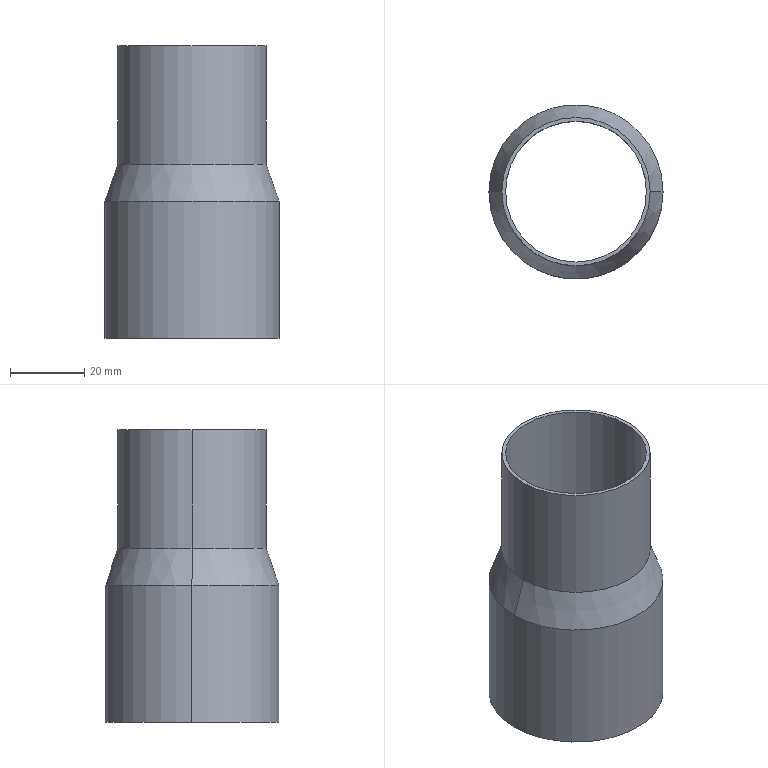Part | SolidWorks | features 3DProfileFeature 2, ICE 2, NetBlend 1, NetBlendCut 1 | 1 solid | 14 faces | box 47 x 47 x 79 mm | volume 10603 mm3 | cylinder 8 | cone 4 | plane 2 | commonest cylinder face diameters 38 x2 40 x2 45 x2 47 x2
STEP:
#1=CARTESIAN_POINT('',(-19.,0.,42.));
#2=VERTEX_POINT('',#1);
#3=CARTESIAN_POINT('',(19.,0.,42.));
#4=VERTEX_POINT('',#3);
#5=CARTESIAN_POINT('',(0.,0.,42.));
#6=DIRECTION('',(0.,0.,1.));
#7=DIRECTION('',(1.,0.,0.));
#8=AXIS2_PLACEMENT_3D('',#5,#6,#7);
#9=CIRCLE('',#8,19.);
#10=EDGE_CURVE('',#2,#4,#9,.T.);
#11=ORIENTED_EDGE('',*,*,#10,.T.);
#12=CARTESIAN_POINT('',(19.,0.,10.));
#13=VERTEX_POINT('',#12);
#14=CARTESIAN_POINT('',(19.,0.,42.));
#15=DIRECTION('',(0.,0.,-1.));
#16=VECTOR('',#15,1000.);
#17=LINE('',#14,#16);
#18=EDGE_CURVE('',#4,#13,#17,.T.);
#19=ORIENTED_EDGE('',*,*,#18,.T.);
#20=CARTESIAN_POINT('',(-19.,0.,10.));
#21=VERTEX_POINT('',#20);
#22=CARTESIAN_POINT('',(0.,0.,10.));
#23=DIRECTION('',(0.,0.,-1.));
#24=DIRECTION('',(1.,0.,0.));
#25=AXIS2_PLACEMENT_3D('',#22,#23,#24);
#26=CIRCLE('',#25,19.);
#27=EDGE_CURVE('',#13,#21,#26,.T.);
#28=ORIENTED_EDGE('',*,*,#27,.T.);
#29=CARTESIAN_POINT('',(-19.,0.,42.));
#30=DIRECTION('',(0.,0.,-1.));
#31=VECTOR('',#30,1000.);
#32=LINE('',#29,#31);
#33=EDGE_CURVE('',#2,#21,#32,.T.);
#34=ORIENTED_EDGE('',*,*,#33,.F.);
#35=EDGE_LOOP('',(#11,#19,#28,#34));
#36=FACE_OUTER_BOUND('',#35,.T.);
#37=CARTESIAN_POINT('',(0.,0.,42.));
#38=DIRECTION('',(0.,0.,-1.));
#39=DIRECTION('',(-1.,0.,0.));
#40=AXIS2_PLACEMENT_3D('',#37,#38,#39);
#41=CYLINDRICAL_SURFACE('',#40,19.);
#42=ADVANCED_FACE('',(#36),#41,.F.);
#43=CARTESIAN_POINT('',(20.,0.,42.));
#44=VERTEX_POINT('',#43);
#45=CARTESIAN_POINT('',(-20.,0.,42.));
#46=VERTEX_POINT('',#45);
#47=CARTESIAN_POINT('',(0.,0.,42.));
#48=DIRECTION('',(0.,0.,1.));
#49=DIRECTION('',(1.,0.,0.));
#50=AXIS2_PLACEMENT_3D('',#47,#48,#49);
#51=CIRCLE('',#50,20.);
#52=EDGE_CURVE('',#44,#46,#51,.T.);
#53=ORIENTED_EDGE('',*,*,#52,.F.);
#54=CARTESIAN_POINT('',(20.,0.,10.));
#55=VERTEX_POINT('',#54);
#56=CARTESIAN_POINT('',(20.,0.,42.));
#57=DIRECTION('',(0.,0.,-1.));
#58=VECTOR('',#57,1000.);
#59=LINE('',#56,#58);
#60=EDGE_CURVE('',#44,#55,#59,.T.);
#61=ORIENTED_EDGE('',*,*,#60,.T.);
#62=CARTESIAN_POINT('',(-20.,0.,10.));
#63=VERTEX_POINT('',#62);
#64=CARTESIAN_POINT('',(0.,0.,10.));
#65=DIRECTION('',(0.,0.,1.));
#66=DIRECTION('',(1.,0.,0.));
#67=AXIS2_PLACEMENT_3D('',#64,#65,#66);
#68=CIRCLE('',#67,20.);
#69=EDGE_CURVE('',#55,#63,#68,.T.);
#70=ORIENTED_EDGE('',*,*,#69,.T.);
#71=CARTESIAN_POINT('',(-20.,0.,42.));
#72=DIRECTION('',(0.,0.,-1.));
#73=VECTOR('',#72,1000.);
#74=LINE('',#71,#73);
#75=EDGE_CURVE('',#46,#63,#74,.T.);
#76=ORIENTED_EDGE('',*,*,#75,.F.);
#77=EDGE_LOOP('',(#53,#61,#70,#76));
#78=FACE_OUTER_BOUND('',#77,.T.);
#79=CARTESIAN_POINT('',(0.,0.,42.));
#80=DIRECTION('',(0.,0.,-1.));
#81=DIRECTION('',(-1.,0.,0.));
#82=AXIS2_PLACEMENT_3D('',#79,#80,#81);
#83=CYLINDRICAL_SURFACE('',#82,20.);
#84=ADVANCED_FACE('',(#78),#83,.T.);
#85=CARTESIAN_POINT('',(22.5,0.,-37.));
#86=VERTEX_POINT('',#85);
#87=CARTESIAN_POINT('',(-22.5,0.,-37.));
#88=VERTEX_POINT('',#87);
#89=CARTESIAN_POINT('',(0.,0.,-37.));
#90=DIRECTION('',(0.,0.,-1.));
#91=DIRECTION('',(-1.,0.,0.));
#92=AXIS2_PLACEMENT_3D('',#89,#90,#91);
#93=CIRCLE('',#92,22.5);
#94=EDGE_CURVE('',#86,#88,#93,.T.);
#95=ORIENTED_EDGE('',*,*,#94,.T.);
#96=CARTESIAN_POINT('',(-22.5,0.,0.));
#97=VERTEX_POINT('',#96);
#98=CARTESIAN_POINT('',(-22.5,0.,-37.));
#99=DIRECTION('',(0.,0.,1.));
#100=VECTOR('',#99,1000.);
#101=LINE('',#98,#100);
#102=EDGE_CURVE('',#88,#97,#101,.T.);
#103=ORIENTED_EDGE('',*,*,#102,.T.);
#104=CARTESIAN_POINT('',(22.5,0.,0.));
#105=VERTEX_POINT('',#104);
#106=CARTESIAN_POINT('',(0.,0.,0.));
#107=DIRECTION('',(0.,0.,-1.));
#108=DIRECTION('',(-1.,0.,0.));
#109=AXIS2_PLACEMENT_3D('',#106,#107,#108);
#110=CIRCLE('',#109,22.5);
#111=EDGE_CURVE('',#105,#97,#110,.T.);
#112=ORIENTED_EDGE('',*,*,#111,.F.);
#113=CARTESIAN_POINT('',(22.5,0.,-37.));
#114=DIRECTION('',(0.,0.,1.));
#115=VECTOR('',#114,1000.);
#116=LINE('',#113,#115);
#117=EDGE_CURVE('',#86,#105,#116,.T.);
#118=ORIENTED_EDGE('',*,*,#117,.F.);
#119=EDGE_LOOP('',(#95,#103,#112,#118));
#120=FACE_OUTER_BOUND('',#119,.T.);
#121=CARTESIAN_POINT('',(0.,0.,-37.));
#122=DIRECTION('',(0.,0.,1.));
#123=DIRECTION('',(1.,0.,0.));
#124=AXIS2_PLACEMENT_3D('',#121,#122,#123);
#125=CYLINDRICAL_SURFACE('',#124,22.5);
#126=ADVANCED_FACE('',(#120),#125,.F.);
#127=CARTESIAN_POINT('',(-23.5,0.,-37.));
#128=VERTEX_POINT('',#127);
#129=CARTESIAN_POINT('',(23.5,0.,-37.));
#130=VERTEX_POINT('',#129);
#131=CARTESIAN_POINT('',(0.,0.,-37.));
#132=DIRECTION('',(0.,0.,-1.));
#133=DIRECTION('',(-1.,0.,0.));
#134=AXIS2_PLACEMENT_3D('',#131,#132,#133);
#135=CIRCLE('',#134,23.5);
#136=EDGE_CURVE('',#128,#130,#135,.T.);
#137=ORIENTED_EDGE('',*,*,#136,.F.);
#138=CARTESIAN_POINT('',(-23.5,0.,0.));
#139=VERTEX_POINT('',#138);
#140=CARTESIAN_POINT('',(-23.5,0.,-37.));
#141=DIRECTION('',(0.,0.,1.));
#142=VECTOR('',#141,1000.);
#143=LINE('',#140,#142);
#144=EDGE_CURVE('',#128,#139,#143,.T.);
#145=ORIENTED_EDGE('',*,*,#144,.T.);
#146=CARTESIAN_POINT('',(23.5,0.,0.));
#147=VERTEX_POINT('',#146);
#148=CARTESIAN_POINT('',(0.,0.,0.));
#149=DIRECTION('',(0.,0.,-1.));
#150=DIRECTION('',(-1.,0.,0.));
#151=AXIS2_PLACEMENT_3D('',#148,#149,#150);
#152=CIRCLE('',#151,23.5);
#153=EDGE_CURVE('',#139,#147,#152,.T.);
#154=ORIENTED_EDGE('',*,*,#153,.T.);
#155=CARTESIAN_POINT('',(23.5,0.,-37.));
#156=DIRECTION('',(0.,0.,1.));
#157=VECTOR('',#156,1000.);
#158=LINE('',#155,#157);
#159=EDGE_CURVE('',#130,#147,#158,.T.);
#160=ORIENTED_EDGE('',*,*,#159,.F.);
#161=EDGE_LOOP('',(#137,#145,#154,#160));
#162=FACE_OUTER_BOUND('',#161,.T.);
#163=CARTESIAN_POINT('',(0.,0.,-37.));
#164=DIRECTION('',(0.,0.,1.));
#165=DIRECTION('',(1.,0.,0.));
#166=AXIS2_PLACEMENT_3D('',#163,#164,#165);
#167=CYLINDRICAL_SURFACE('',#166,23.5);
#168=ADVANCED_FACE('',(#162),#167,.T.);
#169=ORIENTED_EDGE('',*,*,#27,.F.);
#170=CARTESIAN_POINT('',(19.,0.,10.));
#171=DIRECTION('',(0.3304,0.,-0.9439));
#172=VECTOR('',#171,1000.);
#173=LINE('',#170,#172);
#174=EDGE_CURVE('',#13,#105,#173,.T.);
#175=ORIENTED_EDGE('',*,*,#174,.T.);
#176=ORIENTED_EDGE('',*,*,#111,.T.);
#177=CARTESIAN_POINT('',(-19.,0.,10.));
#178=DIRECTION('',(-0.3304,0.,-0.9439));
#179=VECTOR('',#178,1000.);
#180=LINE('',#177,#179);
#181=EDGE_CURVE('',#21,#97,#180,.T.);
#182=ORIENTED_EDGE('',*,*,#181,.F.);
#183=EDGE_LOOP('',(#169,#175,#176,#182));
#184=FACE_OUTER_BOUND('',#183,.T.);
#185=CARTESIAN_POINT('',(0.,0.,10.));
#186=DIRECTION('',(0.,0.,-1.));
#187=DIRECTION('',(-1.,0.,0.));
#188=AXIS2_PLACEMENT_3D('',#185,#186,#187);
#189=CONICAL_SURFACE('',#188,19.,0.3367);
#190=ADVANCED_FACE('',(#184),#189,.F.);
#191=ORIENTED_EDGE('',*,*,#69,.F.);
#192=CARTESIAN_POINT('',(20.,0.,10.));
#193=DIRECTION('',(0.3304,0.,-0.9439));
#194=VECTOR('',#193,1000.);
#195=LINE('',#192,#194);
#196=EDGE_CURVE('',#55,#147,#195,.T.);
#197=ORIENTED_EDGE('',*,*,#196,.T.);
#198=ORIENTED_EDGE('',*,*,#153,.F.);
#199=CARTESIAN_POINT('',(-20.,0.,10.));
#200=DIRECTION('',(-0.3304,0.,-0.9439));
#201=VECTOR('',#200,1000.);
#202=LINE('',#199,#201);
#203=EDGE_CURVE('',#63,#139,#202,.T.);
#204=ORIENTED_EDGE('',*,*,#203,.F.);
#205=EDGE_LOOP('',(#191,#197,#198,#204));
#206=FACE_OUTER_BOUND('',#205,.T.);
#207=CARTESIAN_POINT('',(0.,0.,10.));
#208=DIRECTION('',(0.,0.,-1.));
#209=DIRECTION('',(-1.,0.,0.));
#210=AXIS2_PLACEMENT_3D('',#207,#208,#209);
#211=CONICAL_SURFACE('',#210,20.,0.3367);
#212=ADVANCED_FACE('',(#206),#211,.T.);
#213=ORIENTED_EDGE('',*,*,#196,.F.);
#214=CARTESIAN_POINT('',(0.,0.,10.));
#215=DIRECTION('',(0.,0.,1.));
#216=DIRECTION('',(1.,0.,0.));
#217=AXIS2_PLACEMENT_3D('',#214,#215,#216);
#218=CIRCLE('',#217,20.);
#219=EDGE_CURVE('',#63,#55,#218,.T.);
#220=ORIENTED_EDGE('',*,*,#219,.F.);
#221=ORIENTED_EDGE('',*,*,#203,.T.);
#222=CARTESIAN_POINT('',(0.,0.,0.));
#223=DIRECTION('',(0.,0.,-1.));
#224=DIRECTION('',(-1.,0.,0.));
#225=AXIS2_PLACEMENT_3D('',#222,#223,#224);
#226=CIRCLE('',#225,23.5);
#227=EDGE_CURVE('',#147,#139,#226,.T.);
#228=ORIENTED_EDGE('',*,*,#227,.F.);
#229=EDGE_LOOP('',(#213,#220,#221,#228));
#230=FACE_OUTER_BOUND('',#229,.T.);
#231=CARTESIAN_POINT('',(0.,0.,10.));
#232=DIRECTION('',(0.,0.,-1.));
#233=DIRECTION('',(-1.,0.,0.));
#234=AXIS2_PLACEMENT_3D('',#231,#232,#233);
#235=CONICAL_SURFACE('',#234,20.,0.3367);
#236=ADVANCED_FACE('',(#230),#235,.T.);
#237=ORIENTED_EDGE('',*,*,#174,.F.);
#238=CARTESIAN_POINT('',(0.,0.,10.));
#239=DIRECTION('',(0.,0.,-1.));
#240=DIRECTION('',(1.,0.,0.));
#241=AXIS2_PLACEMENT_3D('',#238,#239,#240);
#242=CIRCLE('',#241,19.);
#243=EDGE_CURVE('',#21,#13,#242,.T.);
#244=ORIENTED_EDGE('',*,*,#243,.F.);
#245=ORIENTED_EDGE('',*,*,#181,.T.);
#246=CARTESIAN_POINT('',(0.,0.,0.));
#247=DIRECTION('',(0.,0.,-1.));
#248=DIRECTION('',(-1.,0.,0.));
#249=AXIS2_PLACEMENT_3D('',#246,#247,#248);
#250=CIRCLE('',#249,22.5);
#251=EDGE_CURVE('',#97,#105,#250,.T.);
#252=ORIENTED_EDGE('',*,*,#251,.T.);
#253=EDGE_LOOP('',(#237,#244,#245,#252));
#254=FACE_OUTER_BOUND('',#253,.T.);
#255=CARTESIAN_POINT('',(0.,0.,10.));
#256=DIRECTION('',(0.,0.,-1.));
#257=DIRECTION('',(-1.,0.,0.));
#258=AXIS2_PLACEMENT_3D('',#255,#256,#257);
#259=CONICAL_SURFACE('',#258,19.,0.3367);
#260=ADVANCED_FACE('',(#254),#259,.F.);
#261=CARTESIAN_POINT('',(0.,0.,-37.));
#262=DIRECTION('',(0.,0.,-1.));
#263=DIRECTION('',(-1.,0.,0.));
#264=AXIS2_PLACEMENT_3D('',#261,#262,#263);
#265=CIRCLE('',#264,23.5);
#266=EDGE_CURVE('',#130,#128,#265,.T.);
#267=ORIENTED_EDGE('',*,*,#266,.T.);
#268=ORIENTED_EDGE('',*,*,#136,.T.);
#269=EDGE_LOOP('',(#267,#268));
#270=FACE_OUTER_BOUND('',#269,.T.);
#271=ORIENTED_EDGE('',*,*,#94,.F.);
#272=CARTESIAN_POINT('',(0.,0.,-37.));
#273=DIRECTION('',(0.,0.,-1.));
#274=DIRECTION('',(-1.,0.,0.));
#275=AXIS2_PLACEMENT_3D('',#272,#273,#274);
#276=CIRCLE('',#275,22.5);
#277=EDGE_CURVE('',#88,#86,#276,.T.);
#278=ORIENTED_EDGE('',*,*,#277,.F.);
#279=EDGE_LOOP('',(#271,#278));
#280=FACE_BOUND('',#279,.T.);
#281=CARTESIAN_POINT('',(0.,0.,-37.));
#282=DIRECTION('',(0.,0.,-1.));
#283=DIRECTION('',(-1.,0.,0.));
#284=AXIS2_PLACEMENT_3D('',#281,#282,#283);
#285=PLANE('',#284);
#286=ADVANCED_FACE('',(#270,#280),#285,.T.);
#287=ORIENTED_EDGE('',*,*,#144,.F.);
#288=ORIENTED_EDGE('',*,*,#266,.F.);
#289=ORIENTED_EDGE('',*,*,#159,.T.);
#290=ORIENTED_EDGE('',*,*,#227,.T.);
#291=EDGE_LOOP('',(#287,#288,#289,#290));
#292=FACE_OUTER_BOUND('',#291,.T.);
#293=CARTESIAN_POINT('',(0.,0.,-37.));
#294=DIRECTION('',(0.,0.,1.));
#295=DIRECTION('',(1.,0.,0.));
#296=AXIS2_PLACEMENT_3D('',#293,#294,#295);
#297=CYLINDRICAL_SURFACE('',#296,23.5);
#298=ADVANCED_FACE('',(#292),#297,.T.);
#299=ORIENTED_EDGE('',*,*,#102,.F.);
#300=ORIENTED_EDGE('',*,*,#277,.T.);
#301=ORIENTED_EDGE('',*,*,#117,.T.);
#302=ORIENTED_EDGE('',*,*,#251,.F.);
#303=EDGE_LOOP('',(#299,#300,#301,#302));
#304=FACE_OUTER_BOUND('',#303,.T.);
#305=CARTESIAN_POINT('',(0.,0.,-37.));
#306=DIRECTION('',(0.,0.,1.));
#307=DIRECTION('',(1.,0.,0.));
#308=AXIS2_PLACEMENT_3D('',#305,#306,#307);
#309=CYLINDRICAL_SURFACE('',#308,22.5);
#310=ADVANCED_FACE('',(#304),#309,.F.);
#311=CARTESIAN_POINT('',(0.,0.,42.));
#312=DIRECTION('',(0.,0.,1.));
#313=DIRECTION('',(1.,0.,0.));
#314=AXIS2_PLACEMENT_3D('',#311,#312,#313);
#315=CIRCLE('',#314,20.);
#316=EDGE_CURVE('',#46,#44,#315,.T.);
#317=ORIENTED_EDGE('',*,*,#316,.T.);
#318=ORIENTED_EDGE('',*,*,#52,.T.);
#319=EDGE_LOOP('',(#317,#318));
#320=FACE_OUTER_BOUND('',#319,.T.);
#321=ORIENTED_EDGE('',*,*,#10,.F.);
#322=CARTESIAN_POINT('',(0.,0.,42.));
#323=DIRECTION('',(0.,0.,1.));
#324=DIRECTION('',(1.,0.,0.));
#325=AXIS2_PLACEMENT_3D('',#322,#323,#324);
#326=CIRCLE('',#325,19.);
#327=EDGE_CURVE('',#4,#2,#326,.T.);
#328=ORIENTED_EDGE('',*,*,#327,.F.);
#329=EDGE_LOOP('',(#321,#328));
#330=FACE_BOUND('',#329,.T.);
#331=CARTESIAN_POINT('',(0.,0.,42.));
#332=DIRECTION('',(0.,0.,1.));
#333=DIRECTION('',(1.,0.,0.));
#334=AXIS2_PLACEMENT_3D('',#331,#332,#333);
#335=PLANE('',#334);
#336=ADVANCED_FACE('',(#320,#330),#335,.T.);
#337=ORIENTED_EDGE('',*,*,#60,.F.);
#338=ORIENTED_EDGE('',*,*,#316,.F.);
#339=ORIENTED_EDGE('',*,*,#75,.T.);
#340=ORIENTED_EDGE('',*,*,#219,.T.);
#341=EDGE_LOOP('',(#337,#338,#339,#340));
#342=FACE_OUTER_BOUND('',#341,.T.);
#343=CARTESIAN_POINT('',(0.,0.,42.));
#344=DIRECTION('',(0.,0.,-1.));
#345=DIRECTION('',(-1.,0.,0.));
#346=AXIS2_PLACEMENT_3D('',#343,#344,#345);
#347=CYLINDRICAL_SURFACE('',#346,20.);
#348=ADVANCED_FACE('',(#342),#347,.T.);
#349=ORIENTED_EDGE('',*,*,#18,.F.);
#350=ORIENTED_EDGE('',*,*,#327,.T.);
#351=ORIENTED_EDGE('',*,*,#33,.T.);
#352=ORIENTED_EDGE('',*,*,#243,.T.);
#353=EDGE_LOOP('',(#349,#350,#351,#352));
#354=FACE_OUTER_BOUND('',#353,.T.);
#355=CARTESIAN_POINT('',(0.,0.,42.));
#356=DIRECTION('',(0.,0.,-1.));
#357=DIRECTION('',(-1.,0.,0.));
#358=AXIS2_PLACEMENT_3D('',#355,#356,#357);
#359=CYLINDRICAL_SURFACE('',#358,19.);
#360=ADVANCED_FACE('',(#354),#359,.F.);
#361=CLOSED_SHELL('',(#42,#84,#126,#168,#190,#212,#236,#260,#286,#298,#310,#336,#348,#360));
#362=MANIFOLD_SOLID_BREP('',#361);
#363=CARTESIAN_POINT('',(0.,0.,0.));
#364=DIRECTION('',(0.,0.,1.));
#365=DIRECTION('',(1.,0.,0.));
#366=AXIS2_PLACEMENT_3D('',#363,#364,#365);
#367=(LENGTH_UNIT()NAMED_UNIT(*)SI_UNIT(.MILLI.,.METRE.));
#368=UNCERTAINTY_MEASURE_WITH_UNIT(LENGTH_MEASURE(0.00001),#367,'','');
#369=(NAMED_UNIT(*)PLANE_ANGLE_UNIT()SI_UNIT($,.RADIAN.));
#370=(NAMED_UNIT(*)SI_UNIT($,.STERADIAN.)SOLID_ANGLE_UNIT());
#371=(GEOMETRIC_REPRESENTATION_CONTEXT(3)GLOBAL_UNCERTAINTY_ASSIGNED_CONTEXT((#368))GLOBAL_UNIT_ASSIGNED_CONTEXT((#367,#369,#370))REPRESENTATION_CONTEXT('',''));
#372=ADVANCED_BREP_SHAPE_REPRESENTATION('',(#362,#366),#371);